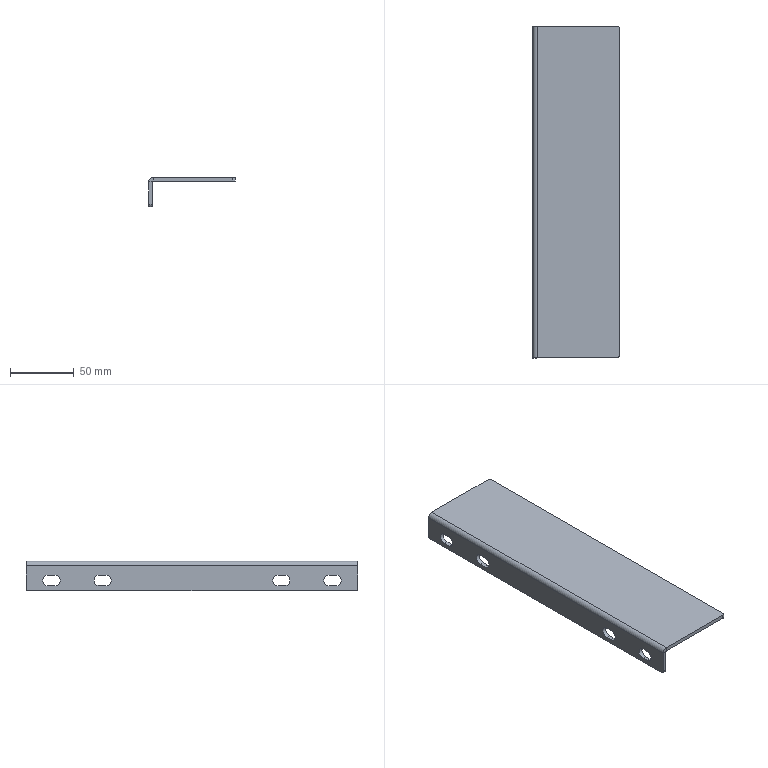Part | STEP file | 1 solid | 34 faces | box 68 x 260 x 23 mm | volume 66736 mm3 | plane 20 | cylinder 14 | commonest cylinder face diameters 8.5 x8 4 x4 1.2 x1 7.2 x1